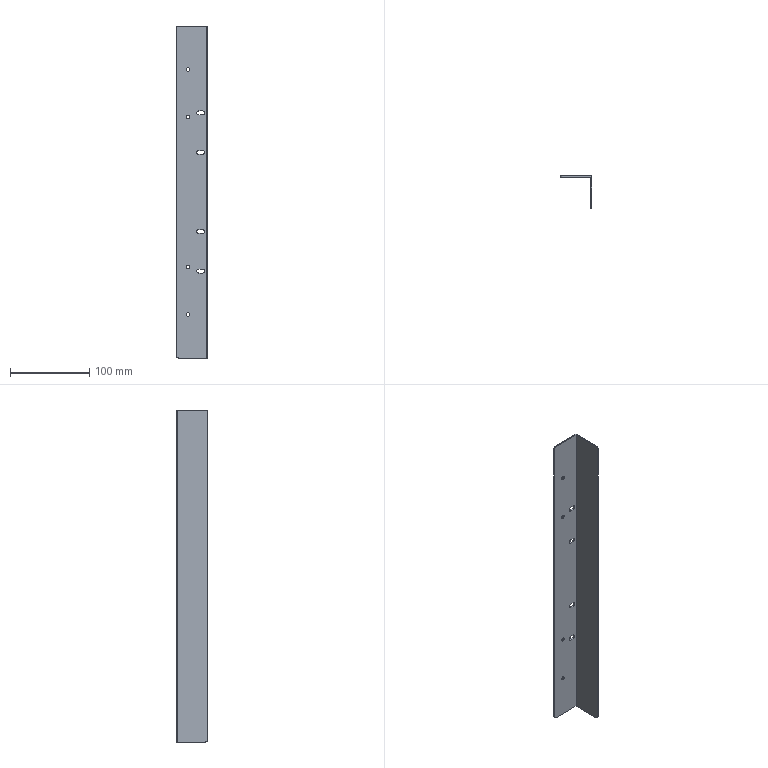Part | SolidWorks | features ICE 3, Cut 2, 3DProfileFeature 1, Extrusion 1, Fillet 1, HoleWzd 1 | 1 solid | 36 faces | box 40 x 40 x 420 mm | volume 49080 mm3 | cylinder 20 | plane 16 | commonest cylinder face diameters 4.5 x8 5 x8 6 x4
STEP:
#1=CARTESIAN_POINT('',(-23.5,20.,157.25));
#2=VERTEX_POINT('',#1);
#3=CARTESIAN_POINT('',(-23.5,20.,152.75));
#4=VERTEX_POINT('',#3);
#5=CARTESIAN_POINT('',(-23.5,20.,155.));
#6=DIRECTION('',(0.,-1.,0.));
#7=DIRECTION('',(0.,0.,-1.));
#8=AXIS2_PLACEMENT_3D('',#5,#6,#7);
#9=CIRCLE('',#8,2.25);
#10=EDGE_CURVE('',#2,#4,#9,.T.);
#11=ORIENTED_EDGE('',*,*,#10,.F.);
#12=CARTESIAN_POINT('',(-23.5,18.5,157.25));
#13=VERTEX_POINT('',#12);
#14=CARTESIAN_POINT('',(-23.5,28.5,157.25));
#15=DIRECTION('',(0.,-1.,0.));
#16=VECTOR('',#15,1000.);
#17=LINE('',#14,#16);
#18=EDGE_CURVE('',#2,#13,#17,.T.);
#19=ORIENTED_EDGE('',*,*,#18,.T.);
#20=CARTESIAN_POINT('',(-23.5,18.5,152.75));
#21=VERTEX_POINT('',#20);
#22=CARTESIAN_POINT('',(-23.5,18.5,155.));
#23=DIRECTION('',(0.,-1.,0.));
#24=DIRECTION('',(0.,0.,1.));
#25=AXIS2_PLACEMENT_3D('',#22,#23,#24);
#26=CIRCLE('',#25,2.25);
#27=EDGE_CURVE('',#13,#21,#26,.T.);
#28=ORIENTED_EDGE('',*,*,#27,.T.);
#29=CARTESIAN_POINT('',(-23.5,28.5,152.75));
#30=DIRECTION('',(0.,-1.,0.));
#31=VECTOR('',#30,1000.);
#32=LINE('',#29,#31);
#33=EDGE_CURVE('',#4,#21,#32,.T.);
#34=ORIENTED_EDGE('',*,*,#33,.F.);
#35=EDGE_LOOP('',(#11,#19,#28,#34));
#36=FACE_OUTER_BOUND('',#35,.T.);
#37=CARTESIAN_POINT('',(-23.5,28.5,155.));
#38=DIRECTION('',(0.,-1.,0.));
#39=DIRECTION('',(0.,0.,-1.));
#40=AXIS2_PLACEMENT_3D('',#37,#38,#39);
#41=CYLINDRICAL_SURFACE('',#40,2.25);
#42=ADVANCED_FACE('',(#36),#41,.F.);
#43=CARTESIAN_POINT('',(-23.5,20.,-152.75));
#44=VERTEX_POINT('',#43);
#45=CARTESIAN_POINT('',(-23.5,20.,-157.25));
#46=VERTEX_POINT('',#45);
#47=CARTESIAN_POINT('',(-23.5,20.,-155.));
#48=DIRECTION('',(0.,-1.,0.));
#49=DIRECTION('',(0.,0.,-1.));
#50=AXIS2_PLACEMENT_3D('',#47,#48,#49);
#51=CIRCLE('',#50,2.25);
#52=EDGE_CURVE('',#44,#46,#51,.T.);
#53=ORIENTED_EDGE('',*,*,#52,.F.);
#54=CARTESIAN_POINT('',(-23.5,18.5,-152.75));
#55=VERTEX_POINT('',#54);
#56=CARTESIAN_POINT('',(-23.5,28.5,-152.75));
#57=DIRECTION('',(0.,-1.,0.));
#58=VECTOR('',#57,1000.);
#59=LINE('',#56,#58);
#60=EDGE_CURVE('',#44,#55,#59,.T.);
#61=ORIENTED_EDGE('',*,*,#60,.T.);
#62=CARTESIAN_POINT('',(-23.5,18.5,-157.25));
#63=VERTEX_POINT('',#62);
#64=CARTESIAN_POINT('',(-23.5,18.5,-155.));
#65=DIRECTION('',(0.,-1.,0.));
#66=DIRECTION('',(0.,0.,-1.));
#67=AXIS2_PLACEMENT_3D('',#64,#65,#66);
#68=CIRCLE('',#67,2.25);
#69=EDGE_CURVE('',#55,#63,#68,.T.);
#70=ORIENTED_EDGE('',*,*,#69,.T.);
#71=CARTESIAN_POINT('',(-23.5,28.5,-157.25));
#72=DIRECTION('',(0.,-1.,0.));
#73=VECTOR('',#72,1000.);
#74=LINE('',#71,#73);
#75=EDGE_CURVE('',#46,#63,#74,.T.);
#76=ORIENTED_EDGE('',*,*,#75,.F.);
#77=EDGE_LOOP('',(#53,#61,#70,#76));
#78=FACE_OUTER_BOUND('',#77,.T.);
#79=CARTESIAN_POINT('',(-23.5,28.5,-155.));
#80=DIRECTION('',(0.,-1.,0.));
#81=DIRECTION('',(0.,0.,-1.));
#82=AXIS2_PLACEMENT_3D('',#79,#80,#81);
#83=CYLINDRICAL_SURFACE('',#82,2.25);
#84=ADVANCED_FACE('',(#78),#83,.F.);
#85=CARTESIAN_POINT('',(-23.5,18.5,-92.75));
#86=VERTEX_POINT('',#85);
#87=CARTESIAN_POINT('',(-23.5,18.5,-97.25));
#88=VERTEX_POINT('',#87);
#89=CARTESIAN_POINT('',(-23.5,18.5,-95.));
#90=DIRECTION('',(0.,-1.,0.));
#91=DIRECTION('',(0.,0.,-1.));
#92=AXIS2_PLACEMENT_3D('',#89,#90,#91);
#93=CIRCLE('',#92,2.25);
#94=EDGE_CURVE('',#86,#88,#93,.T.);
#95=ORIENTED_EDGE('',*,*,#94,.T.);
#96=CARTESIAN_POINT('',(-23.5,20.,-97.25));
#97=VERTEX_POINT('',#96);
#98=CARTESIAN_POINT('',(-23.5,10.,-97.25));
#99=DIRECTION('',(0.,1.,0.));
#100=VECTOR('',#99,1000.);
#101=LINE('',#98,#100);
#102=EDGE_CURVE('',#88,#97,#101,.T.);
#103=ORIENTED_EDGE('',*,*,#102,.T.);
#104=CARTESIAN_POINT('',(-23.5,20.,-92.75));
#105=VERTEX_POINT('',#104);
#106=CARTESIAN_POINT('',(-23.5,20.,-95.));
#107=DIRECTION('',(0.,1.,0.));
#108=DIRECTION('',(0.,0.,-1.));
#109=AXIS2_PLACEMENT_3D('',#106,#107,#108);
#110=CIRCLE('',#109,2.25);
#111=EDGE_CURVE('',#97,#105,#110,.T.);
#112=ORIENTED_EDGE('',*,*,#111,.T.);
#113=CARTESIAN_POINT('',(-23.5,10.,-92.75));
#114=DIRECTION('',(0.,1.,0.));
#115=VECTOR('',#114,1000.);
#116=LINE('',#113,#115);
#117=EDGE_CURVE('',#86,#105,#116,.T.);
#118=ORIENTED_EDGE('',*,*,#117,.F.);
#119=EDGE_LOOP('',(#95,#103,#112,#118));
#120=FACE_OUTER_BOUND('',#119,.T.);
#121=CARTESIAN_POINT('',(-23.5,10.,-95.));
#122=DIRECTION('',(0.,1.,0.));
#123=DIRECTION('',(0.,0.,1.));
#124=AXIS2_PLACEMENT_3D('',#121,#122,#123);
#125=CYLINDRICAL_SURFACE('',#124,2.25);
#126=ADVANCED_FACE('',(#120),#125,.F.);
#127=CARTESIAN_POINT('',(-23.5,18.5,97.25));
#128=VERTEX_POINT('',#127);
#129=CARTESIAN_POINT('',(-23.5,18.5,92.75));
#130=VERTEX_POINT('',#129);
#131=CARTESIAN_POINT('',(-23.5,18.5,95.));
#132=DIRECTION('',(0.,-1.,0.));
#133=DIRECTION('',(0.,0.,-1.));
#134=AXIS2_PLACEMENT_3D('',#131,#132,#133);
#135=CIRCLE('',#134,2.25);
#136=EDGE_CURVE('',#128,#130,#135,.T.);
#137=ORIENTED_EDGE('',*,*,#136,.T.);
#138=CARTESIAN_POINT('',(-23.5,20.,92.75));
#139=VERTEX_POINT('',#138);
#140=CARTESIAN_POINT('',(-23.5,10.,92.75));
#141=DIRECTION('',(0.,1.,0.));
#142=VECTOR('',#141,1000.);
#143=LINE('',#140,#142);
#144=EDGE_CURVE('',#130,#139,#143,.T.);
#145=ORIENTED_EDGE('',*,*,#144,.T.);
#146=CARTESIAN_POINT('',(-23.5,20.,97.25));
#147=VERTEX_POINT('',#146);
#148=CARTESIAN_POINT('',(-23.5,20.,95.));
#149=DIRECTION('',(0.,1.,0.));
#150=DIRECTION('',(0.,0.,1.));
#151=AXIS2_PLACEMENT_3D('',#148,#149,#150);
#152=CIRCLE('',#151,2.25);
#153=EDGE_CURVE('',#139,#147,#152,.T.);
#154=ORIENTED_EDGE('',*,*,#153,.T.);
#155=CARTESIAN_POINT('',(-23.5,10.,97.25));
#156=DIRECTION('',(0.,1.,0.));
#157=VECTOR('',#156,1000.);
#158=LINE('',#155,#157);
#159=EDGE_CURVE('',#128,#147,#158,.T.);
#160=ORIENTED_EDGE('',*,*,#159,.F.);
#161=EDGE_LOOP('',(#137,#145,#154,#160));
#162=FACE_OUTER_BOUND('',#161,.T.);
#163=CARTESIAN_POINT('',(-23.5,10.,95.));
#164=DIRECTION('',(0.,1.,0.));
#165=DIRECTION('',(0.,0.,1.));
#166=AXIS2_PLACEMENT_3D('',#163,#164,#165);
#167=CYLINDRICAL_SURFACE('',#166,2.25);
#168=ADVANCED_FACE('',(#162),#167,.F.);
#169=CARTESIAN_POINT('',(1.5,20.,210.));
#170=VERTEX_POINT('',#169);
#171=CARTESIAN_POINT('',(-35.5,20.,210.));
#172=VERTEX_POINT('',#171);
#173=CARTESIAN_POINT('',(1.5,20.,210.));
#174=DIRECTION('',(-1.,0.,0.));
#175=VECTOR('',#174,1000.);
#176=LINE('',#173,#175);
#177=EDGE_CURVE('',#170,#172,#176,.T.);
#178=ORIENTED_EDGE('',*,*,#177,.T.);
#179=CARTESIAN_POINT('',(-35.5,18.5,210.));
#180=VERTEX_POINT('',#179);
#181=CARTESIAN_POINT('',(-35.5,20.,210.));
#182=DIRECTION('',(0.,-1.,0.));
#183=VECTOR('',#182,1000.);
#184=LINE('',#181,#183);
#185=EDGE_CURVE('',#172,#180,#184,.T.);
#186=ORIENTED_EDGE('',*,*,#185,.T.);
#187=CARTESIAN_POINT('',(0.,18.5,210.));
#188=VERTEX_POINT('',#187);
#189=CARTESIAN_POINT('',(-38.5,18.5,210.));
#190=DIRECTION('',(1.,0.,0.));
#191=VECTOR('',#190,1000.);
#192=LINE('',#189,#191);
#193=EDGE_CURVE('',#180,#188,#192,.T.);
#194=ORIENTED_EDGE('',*,*,#193,.T.);
#195=CARTESIAN_POINT('',(0.,-17.,210.));
#196=VERTEX_POINT('',#195);
#197=CARTESIAN_POINT('',(0.,20.,210.));
#198=DIRECTION('',(0.,-1.,0.));
#199=VECTOR('',#198,1000.);
#200=LINE('',#197,#199);
#201=EDGE_CURVE('',#188,#196,#200,.T.);
#202=ORIENTED_EDGE('',*,*,#201,.T.);
#203=CARTESIAN_POINT('',(1.5,-17.,210.));
#204=VERTEX_POINT('',#203);
#205=CARTESIAN_POINT('',(1.5,-17.,210.));
#206=DIRECTION('',(1.,0.,0.));
#207=VECTOR('',#206,1000.);
#208=LINE('',#205,#207);
#209=EDGE_CURVE('',#196,#204,#208,.T.);
#210=ORIENTED_EDGE('',*,*,#209,.T.);
#211=CARTESIAN_POINT('',(1.5,20.,210.));
#212=DIRECTION('',(0.,-1.,0.));
#213=VECTOR('',#212,1000.);
#214=LINE('',#211,#213);
#215=EDGE_CURVE('',#170,#204,#214,.T.);
#216=ORIENTED_EDGE('',*,*,#215,.F.);
#217=EDGE_LOOP('',(#178,#186,#194,#202,#210,#216));
#218=FACE_OUTER_BOUND('',#217,.T.);
#219=CARTESIAN_POINT('',(1.5,20.,210.));
#220=DIRECTION('',(0.,0.,-1.));
#221=DIRECTION('',(-1.,0.,0.));
#222=AXIS2_PLACEMENT_3D('',#219,#220,#221);
#223=PLANE('',#222);
#224=ADVANCED_FACE('',(#218),#223,.F.);
#225=CARTESIAN_POINT('',(1.5,-20.,207.));
#226=VERTEX_POINT('',#225);
#227=CARTESIAN_POINT('',(1.5,-20.,-207.));
#228=VERTEX_POINT('',#227);
#229=CARTESIAN_POINT('',(1.5,-20.,210.));
#230=DIRECTION('',(0.,0.,-1.));
#231=VECTOR('',#230,1000.);
#232=LINE('',#229,#231);
#233=EDGE_CURVE('',#226,#228,#232,.T.);
#234=ORIENTED_EDGE('',*,*,#233,.F.);
#235=CARTESIAN_POINT('',(0.,-20.,207.));
#236=VERTEX_POINT('',#235);
#237=CARTESIAN_POINT('',(1.5,-20.,207.));
#238=DIRECTION('',(-1.,0.,0.));
#239=VECTOR('',#238,1000.);
#240=LINE('',#237,#239);
#241=EDGE_CURVE('',#226,#236,#240,.T.);
#242=ORIENTED_EDGE('',*,*,#241,.T.);
#243=CARTESIAN_POINT('',(0.,-20.,-207.));
#244=VERTEX_POINT('',#243);
#245=CARTESIAN_POINT('',(0.,-20.,210.));
#246=DIRECTION('',(0.,0.,-1.));
#247=VECTOR('',#246,1000.);
#248=LINE('',#245,#247);
#249=EDGE_CURVE('',#236,#244,#248,.T.);
#250=ORIENTED_EDGE('',*,*,#249,.T.);
#251=CARTESIAN_POINT('',(1.5,-20.,-207.));
#252=DIRECTION('',(1.,0.,0.));
#253=VECTOR('',#252,1000.);
#254=LINE('',#251,#253);
#255=EDGE_CURVE('',#244,#228,#254,.T.);
#256=ORIENTED_EDGE('',*,*,#255,.T.);
#257=EDGE_LOOP('',(#234,#242,#250,#256));
#258=FACE_OUTER_BOUND('',#257,.T.);
#259=CARTESIAN_POINT('',(1.5,-20.,210.));
#260=DIRECTION('',(0.,1.,0.));
#261=DIRECTION('',(0.,0.,1.));
#262=AXIS2_PLACEMENT_3D('',#259,#260,#261);
#263=PLANE('',#262);
#264=ADVANCED_FACE('',(#258),#263,.F.);
#265=CARTESIAN_POINT('',(-35.5,18.5,-210.));
#266=VERTEX_POINT('',#265);
#267=CARTESIAN_POINT('',(0.,18.5,-210.));
#268=VERTEX_POINT('',#267);
#269=CARTESIAN_POINT('',(-38.5,18.5,-210.));
#270=DIRECTION('',(1.,0.,0.));
#271=VECTOR('',#270,1000.);
#272=LINE('',#269,#271);
#273=EDGE_CURVE('',#266,#268,#272,.T.);
#274=ORIENTED_EDGE('',*,*,#273,.F.);
#275=CARTESIAN_POINT('',(-35.5,20.,-210.));
#276=VERTEX_POINT('',#275);
#277=CARTESIAN_POINT('',(-35.5,20.,-210.));
#278=DIRECTION('',(0.,1.,0.));
#279=VECTOR('',#278,1000.);
#280=LINE('',#277,#279);
#281=EDGE_CURVE('',#266,#276,#280,.T.);
#282=ORIENTED_EDGE('',*,*,#281,.T.);
#283=CARTESIAN_POINT('',(1.5,20.,-210.));
#284=VERTEX_POINT('',#283);
#285=CARTESIAN_POINT('',(1.5,20.,-210.));
#286=DIRECTION('',(-1.,0.,0.));
#287=VECTOR('',#286,1000.);
#288=LINE('',#285,#287);
#289=EDGE_CURVE('',#284,#276,#288,.T.);
#290=ORIENTED_EDGE('',*,*,#289,.F.);
#291=CARTESIAN_POINT('',(1.5,-17.,-210.));
#292=VERTEX_POINT('',#291);
#293=CARTESIAN_POINT('',(1.5,20.,-210.));
#294=DIRECTION('',(0.,1.,0.));
#295=VECTOR('',#294,1000.);
#296=LINE('',#293,#295);
#297=EDGE_CURVE('',#292,#284,#296,.T.);
#298=ORIENTED_EDGE('',*,*,#297,.F.);
#299=CARTESIAN_POINT('',(0.,-17.,-210.));
#300=VERTEX_POINT('',#299);
#301=CARTESIAN_POINT('',(1.5,-17.,-210.));
#302=DIRECTION('',(-1.,0.,0.));
#303=VECTOR('',#302,1000.);
#304=LINE('',#301,#303);
#305=EDGE_CURVE('',#292,#300,#304,.T.);
#306=ORIENTED_EDGE('',*,*,#305,.T.);
#307=CARTESIAN_POINT('',(0.,20.,-210.));
#308=DIRECTION('',(0.,1.,0.));
#309=VECTOR('',#308,1000.);
#310=LINE('',#307,#309);
#311=EDGE_CURVE('',#300,#268,#310,.T.);
#312=ORIENTED_EDGE('',*,*,#311,.T.);
#313=EDGE_LOOP('',(#274,#282,#290,#298,#306,#312));
#314=FACE_OUTER_BOUND('',#313,.T.);
#315=CARTESIAN_POINT('',(1.5,20.,-210.));
#316=DIRECTION('',(0.,0.,1.));
#317=DIRECTION('',(1.,0.,0.));
#318=AXIS2_PLACEMENT_3D('',#315,#316,#317);
#319=PLANE('',#318);
#320=ADVANCED_FACE('',(#314),#319,.F.);
#321=CARTESIAN_POINT('',(-5.,20.,-102.5));
#322=VERTEX_POINT('',#321);
#323=CARTESIAN_POINT('',(-10.,20.,-102.5));
#324=VERTEX_POINT('',#323);
#325=CARTESIAN_POINT('',(-5.,20.,-102.5));
#326=DIRECTION('',(-1.,0.,0.));
#327=VECTOR('',#326,1000.);
#328=LINE('',#325,#327);
#329=EDGE_CURVE('',#322,#324,#328,.T.);
#330=ORIENTED_EDGE('',*,*,#329,.F.);
#331=CARTESIAN_POINT('',(-5.,20.,-97.5));
#332=VERTEX_POINT('',#331);
#333=CARTESIAN_POINT('',(-5.,20.,-100.));
#334=DIRECTION('',(0.,1.,0.));
#335=DIRECTION('',(0.,0.,1.));
#336=AXIS2_PLACEMENT_3D('',#333,#334,#335);
#337=CIRCLE('',#336,2.5);
#338=EDGE_CURVE('',#332,#322,#337,.T.);
#339=ORIENTED_EDGE('',*,*,#338,.F.);
#340=CARTESIAN_POINT('',(-10.,20.,-97.5));
#341=VERTEX_POINT('',#340);
#342=CARTESIAN_POINT('',(-5.,20.,-97.5));
#343=DIRECTION('',(1.,0.,0.));
#344=VECTOR('',#343,1000.);
#345=LINE('',#342,#344);
#346=EDGE_CURVE('',#341,#332,#345,.T.);
#347=ORIENTED_EDGE('',*,*,#346,.F.);
#348=CARTESIAN_POINT('',(-10.,20.,-100.));
#349=DIRECTION('',(0.,1.,0.));
#350=DIRECTION('',(0.,0.,1.));
#351=AXIS2_PLACEMENT_3D('',#348,#349,#350);
#352=CIRCLE('',#351,2.5);
#353=EDGE_CURVE('',#324,#341,#352,.T.);
#354=ORIENTED_EDGE('',*,*,#353,.F.);
#355=EDGE_LOOP('',(#330,#339,#347,#354));
#356=FACE_BOUND('',#355,.T.);
#357=CARTESIAN_POINT('',(-5.,20.,47.5));
#358=VERTEX_POINT('',#357);
#359=CARTESIAN_POINT('',(-10.,20.,47.5));
#360=VERTEX_POINT('',#359);
#361=CARTESIAN_POINT('',(-5.,20.,47.5));
#362=DIRECTION('',(-1.,0.,0.));
#363=VECTOR('',#362,1000.);
#364=LINE('',#361,#363);
#365=EDGE_CURVE('',#358,#360,#364,.T.);
#366=ORIENTED_EDGE('',*,*,#365,.F.);
#367=CARTESIAN_POINT('',(-5.,20.,52.5));
#368=VERTEX_POINT('',#367);
#369=CARTESIAN_POINT('',(-5.,20.,50.));
#370=DIRECTION('',(0.,1.,0.));
#371=DIRECTION('',(0.,0.,1.));
#372=AXIS2_PLACEMENT_3D('',#369,#370,#371);
#373=CIRCLE('',#372,2.5);
#374=EDGE_CURVE('',#368,#358,#373,.T.);
#375=ORIENTED_EDGE('',*,*,#374,.F.);
#376=CARTESIAN_POINT('',(-10.,20.,52.5));
#377=VERTEX_POINT('',#376);
#378=CARTESIAN_POINT('',(-5.,20.,52.5));
#379=DIRECTION('',(1.,0.,0.));
#380=VECTOR('',#379,1000.);
#381=LINE('',#378,#380);
#382=EDGE_CURVE('',#377,#368,#381,.T.);
#383=ORIENTED_EDGE('',*,*,#382,.F.);
#384=CARTESIAN_POINT('',(-10.,20.,50.));
#385=DIRECTION('',(0.,1.,0.));
#386=DIRECTION('',(0.,0.,1.));
#387=AXIS2_PLACEMENT_3D('',#384,#385,#386);
#388=CIRCLE('',#387,2.5);
#389=EDGE_CURVE('',#360,#377,#388,.T.);
#390=ORIENTED_EDGE('',*,*,#389,.F.);
#391=EDGE_LOOP('',(#366,#375,#383,#390));
#392=FACE_BOUND('',#391,.T.);
#393=CARTESIAN_POINT('',(-5.,20.,-52.5));
#394=VERTEX_POINT('',#393);
#395=CARTESIAN_POINT('',(-10.,20.,-52.5));
#396=VERTEX_POINT('',#395);
#397=CARTESIAN_POINT('',(-5.,20.,-52.5));
#398=DIRECTION('',(-1.,0.,0.));
#399=VECTOR('',#398,1000.);
#400=LINE('',#397,#399);
#401=EDGE_CURVE('',#394,#396,#400,.T.);
#402=ORIENTED_EDGE('',*,*,#401,.F.);
#403=CARTESIAN_POINT('',(-5.,20.,-47.5));
#404=VERTEX_POINT('',#403);
#405=CARTESIAN_POINT('',(-5.,20.,-50.));
#406=DIRECTION('',(0.,1.,0.));
#407=DIRECTION('',(0.,0.,1.));
#408=AXIS2_PLACEMENT_3D('',#405,#406,#407);
#409=CIRCLE('',#408,2.5);
#410=EDGE_CURVE('',#404,#394,#409,.T.);
#411=ORIENTED_EDGE('',*,*,#410,.F.);
#412=CARTESIAN_POINT('',(-10.,20.,-47.5));
#413=VERTEX_POINT('',#412);
#414=CARTESIAN_POINT('',(-5.,20.,-47.5));
#415=DIRECTION('',(1.,0.,0.));
#416=VECTOR('',#415,1000.);
#417=LINE('',#414,#416);
#418=EDGE_CURVE('',#413,#404,#417,.T.);
#419=ORIENTED_EDGE('',*,*,#418,.F.);
#420=CARTESIAN_POINT('',(-10.,20.,-50.));
#421=DIRECTION('',(0.,1.,0.));
#422=DIRECTION('',(0.,0.,1.));
#423=AXIS2_PLACEMENT_3D('',#420,#421,#422);
#424=CIRCLE('',#423,2.5);
#425=EDGE_CURVE('',#396,#413,#424,.T.);
#426=ORIENTED_EDGE('',*,*,#425,.F.);
#427=EDGE_LOOP('',(#402,#411,#419,#426));
#428=FACE_BOUND('',#427,.T.);
#429=CARTESIAN_POINT('',(-10.,20.,102.5));
#430=VERTEX_POINT('',#429);
#431=CARTESIAN_POINT('',(-5.,20.,102.5));
#432=VERTEX_POINT('',#431);
#433=CARTESIAN_POINT('',(-10.,20.,102.5));
#434=DIRECTION('',(1.,0.,0.));
#435=VECTOR('',#434,1000.);
#436=LINE('',#433,#435);
#437=EDGE_CURVE('',#430,#432,#436,.T.);
#438=ORIENTED_EDGE('',*,*,#437,.F.);
#439=CARTESIAN_POINT('',(-10.,20.,97.5));
#440=VERTEX_POINT('',#439);
#441=CARTESIAN_POINT('',(-10.,20.,100.));
#442=DIRECTION('',(0.,1.,0.));
#443=DIRECTION('',(0.,0.,1.));
#444=AXIS2_PLACEMENT_3D('',#441,#442,#443);
#445=CIRCLE('',#444,2.5);
#446=EDGE_CURVE('',#440,#430,#445,.T.);
#447=ORIENTED_EDGE('',*,*,#446,.F.);
#448=CARTESIAN_POINT('',(-5.,20.,97.5));
#449=VERTEX_POINT('',#448);
#450=CARTESIAN_POINT('',(-10.,20.,97.5));
#451=DIRECTION('',(-1.,0.,0.));
#452=VECTOR('',#451,1000.);
#453=LINE('',#450,#452);
#454=EDGE_CURVE('',#449,#440,#453,.T.);
#455=ORIENTED_EDGE('',*,*,#454,.F.);
#456=CARTESIAN_POINT('',(-5.,20.,100.));
#457=DIRECTION('',(0.,1.,0.));
#458=DIRECTION('',(0.,0.,1.));
#459=AXIS2_PLACEMENT_3D('',#456,#457,#458);
#460=CIRCLE('',#459,2.5);
#461=EDGE_CURVE('',#432,#449,#460,.T.);
#462=ORIENTED_EDGE('',*,*,#461,.F.);
#463=EDGE_LOOP('',(#438,#447,#455,#462));
#464=FACE_BOUND('',#463,.T.);
#465=CARTESIAN_POINT('',(-23.5,20.,155.));
#466=DIRECTION('',(0.,-1.,0.));
#467=DIRECTION('',(0.,0.,-1.));
#468=AXIS2_PLACEMENT_3D('',#465,#466,#467);
#469=CIRCLE('',#468,2.25);
#470=EDGE_CURVE('',#4,#2,#469,.T.);
#471=ORIENTED_EDGE('',*,*,#470,.T.);
#472=ORIENTED_EDGE('',*,*,#10,.T.);
#473=EDGE_LOOP('',(#471,#472));
#474=FACE_BOUND('',#473,.T.);
#475=CARTESIAN_POINT('',(-23.5,20.,-155.));
#476=DIRECTION('',(0.,-1.,0.));
#477=DIRECTION('',(0.,0.,-1.));
#478=AXIS2_PLACEMENT_3D('',#475,#476,#477);
#479=CIRCLE('',#478,2.25);
#480=EDGE_CURVE('',#46,#44,#479,.T.);
#481=ORIENTED_EDGE('',*,*,#480,.T.);
#482=ORIENTED_EDGE('',*,*,#52,.T.);
#483=EDGE_LOOP('',(#481,#482));
#484=FACE_BOUND('',#483,.T.);
#485=CARTESIAN_POINT('',(-23.5,20.,-95.));
#486=DIRECTION('',(0.,1.,0.));
#487=DIRECTION('',(0.,0.,-1.));
#488=AXIS2_PLACEMENT_3D('',#485,#486,#487);
#489=CIRCLE('',#488,2.25);
#490=EDGE_CURVE('',#105,#97,#489,.T.);
#491=ORIENTED_EDGE('',*,*,#490,.F.);
#492=ORIENTED_EDGE('',*,*,#111,.F.);
#493=EDGE_LOOP('',(#491,#492));
#494=FACE_BOUND('',#493,.T.);
#495=CARTESIAN_POINT('',(-23.5,20.,95.));
#496=DIRECTION('',(0.,1.,0.));
#497=DIRECTION('',(0.,0.,1.));
#498=AXIS2_PLACEMENT_3D('',#495,#496,#497);
#499=CIRCLE('',#498,2.25);
#500=EDGE_CURVE('',#147,#139,#499,.T.);
#501=ORIENTED_EDGE('',*,*,#500,.F.);
#502=ORIENTED_EDGE('',*,*,#153,.F.);
#503=EDGE_LOOP('',(#501,#502));
#504=FACE_BOUND('',#503,.T.);
#505=CARTESIAN_POINT('',(-38.5,20.,-207.));
#506=VERTEX_POINT('',#505);
#507=CARTESIAN_POINT('',(-38.5,20.,207.));
#508=VERTEX_POINT('',#507);
#509=CARTESIAN_POINT('',(-38.5,20.,210.));
#510=DIRECTION('',(0.,0.,1.));
#511=VECTOR('',#510,1000.);
#512=LINE('',#509,#511);
#513=EDGE_CURVE('',#506,#508,#512,.T.);
#514=ORIENTED_EDGE('',*,*,#513,.T.);
#515=CARTESIAN_POINT('',(-35.5,20.,207.));
#516=DIRECTION('',(0.,1.,0.));
#517=DIRECTION('',(0.,0.,-1.));
#518=AXIS2_PLACEMENT_3D('',#515,#516,#517);
#519=CIRCLE('',#518,3.);
#520=EDGE_CURVE('',#508,#172,#519,.T.);
#521=ORIENTED_EDGE('',*,*,#520,.T.);
#522=ORIENTED_EDGE('',*,*,#177,.F.);
#523=CARTESIAN_POINT('',(1.5,20.,210.));
#524=DIRECTION('',(0.,0.,1.));
#525=VECTOR('',#524,1000.);
#526=LINE('',#523,#525);
#527=EDGE_CURVE('',#284,#170,#526,.T.);
#528=ORIENTED_EDGE('',*,*,#527,.F.);
#529=ORIENTED_EDGE('',*,*,#289,.T.);
#530=CARTESIAN_POINT('',(-35.5,20.,-207.));
#531=DIRECTION('',(0.,1.,0.));
#532=DIRECTION('',(0.,0.,-1.));
#533=AXIS2_PLACEMENT_3D('',#530,#531,#532);
#534=CIRCLE('',#533,3.);
#535=EDGE_CURVE('',#276,#506,#534,.T.);
#536=ORIENTED_EDGE('',*,*,#535,.T.);
#537=EDGE_LOOP('',(#514,#521,#522,#528,#529,#536));
#538=FACE_OUTER_BOUND('',#537,.T.);
#539=CARTESIAN_POINT('',(1.5,20.,210.));
#540=DIRECTION('',(0.,-1.,0.));
#541=DIRECTION('',(0.,0.,-1.));
#542=AXIS2_PLACEMENT_3D('',#539,#540,#541);
#543=PLANE('',#542);
#544=ADVANCED_FACE('',(#356,#392,#428,#464,#474,#484,#494,#504,#538),#543,.F.);
#545=ORIENTED_EDGE('',*,*,#215,.T.);
#546=CARTESIAN_POINT('',(1.5,-17.,207.));
#547=DIRECTION('',(1.,0.,0.));
#548=DIRECTION('',(0.,0.,-1.));
#549=AXIS2_PLACEMENT_3D('',#546,#547,#548);
#550=CIRCLE('',#549,3.);
#551=EDGE_CURVE('',#204,#226,#550,.T.);
#552=ORIENTED_EDGE('',*,*,#551,.T.);
#553=ORIENTED_EDGE('',*,*,#233,.T.);
#554=CARTESIAN_POINT('',(1.5,-17.,-207.));
#555=DIRECTION('',(1.,0.,0.));
#556=DIRECTION('',(0.,0.,-1.));
#557=AXIS2_PLACEMENT_3D('',#554,#555,#556);
#558=CIRCLE('',#557,3.);
#559=EDGE_CURVE('',#228,#292,#558,.T.);
#560=ORIENTED_EDGE('',*,*,#559,.T.);
#561=ORIENTED_EDGE('',*,*,#297,.T.);
#562=ORIENTED_EDGE('',*,*,#527,.T.);
#563=EDGE_LOOP('',(#545,#552,#553,#560,#561,#562));
#564=FACE_OUTER_BOUND('',#563,.T.);
#565=CARTESIAN_POINT('',(1.5,-20.,210.));
#566=DIRECTION('',(1.,0.,0.));
#567=DIRECTION('',(0.,0.,-1.));
#568=AXIS2_PLACEMENT_3D('',#565,#566,#567);
#569=PLANE('',#568);
#570=ADVANCED_FACE('',(#564),#569,.T.);
#571=ORIENTED_EDGE('',*,*,#249,.F.);
#572=CARTESIAN_POINT('',(0.,-17.,207.));
#573=DIRECTION('',(-1.,0.,0.));
#574=DIRECTION('',(0.,0.,-1.));
#575=AXIS2_PLACEMENT_3D('',#572,#573,#574);
#576=CIRCLE('',#575,3.);
#577=EDGE_CURVE('',#236,#196,#576,.T.);
#578=ORIENTED_EDGE('',*,*,#577,.T.);
#579=ORIENTED_EDGE('',*,*,#201,.F.);
#580=CARTESIAN_POINT('',(0.,18.5,210.));
#581=DIRECTION('',(0.,0.,-1.));
#582=VECTOR('',#581,1000.);
#583=LINE('',#580,#582);
#584=EDGE_CURVE('',#188,#268,#583,.T.);
#585=ORIENTED_EDGE('',*,*,#584,.T.);
#586=ORIENTED_EDGE('',*,*,#311,.F.);
#587=CARTESIAN_POINT('',(0.,-17.,-207.));
#588=DIRECTION('',(-1.,0.,0.));
#589=DIRECTION('',(0.,0.,-1.));
#590=AXIS2_PLACEMENT_3D('',#587,#588,#589);
#591=CIRCLE('',#590,3.);
#592=EDGE_CURVE('',#300,#244,#591,.T.);
#593=ORIENTED_EDGE('',*,*,#592,.T.);
#594=EDGE_LOOP('',(#571,#578,#579,#585,#586,#593));
#595=FACE_OUTER_BOUND('',#594,.T.);
#596=CARTESIAN_POINT('',(0.,-20.,210.));
#597=DIRECTION('',(1.,0.,0.));
#598=DIRECTION('',(0.,0.,-1.));
#599=AXIS2_PLACEMENT_3D('',#596,#597,#598);
#600=PLANE('',#599);
#601=ADVANCED_FACE('',(#595),#600,.F.);
#602=CARTESIAN_POINT('',(-5.,18.5,-102.5));
#603=VERTEX_POINT('',#602);
#604=CARTESIAN_POINT('',(-5.,18.5,-97.5));
#605=VERTEX_POINT('',#604);
#606=CARTESIAN_POINT('',(-5.,18.5,-100.));
#607=DIRECTION('',(0.,-1.,0.));
#608=DIRECTION('',(0.,0.,-1.));
#609=AXIS2_PLACEMENT_3D('',#606,#607,#608);
#610=CIRCLE('',#609,2.5);
#611=EDGE_CURVE('',#603,#605,#610,.T.);
#612=ORIENTED_EDGE('',*,*,#611,.F.);
#613=CARTESIAN_POINT('',(-10.,18.5,-102.5));
#614=VERTEX_POINT('',#613);
#615=CARTESIAN_POINT('',(-38.5,18.5,-102.5));
#616=DIRECTION('',(1.,0.,0.));
#617=VECTOR('',#616,1000.);
#618=LINE('',#615,#617);
#619=EDGE_CURVE('',#614,#603,#618,.T.);
#620=ORIENTED_EDGE('',*,*,#619,.F.);
#621=CARTESIAN_POINT('',(-10.,18.5,-97.5));
#622=VERTEX_POINT('',#621);
#623=CARTESIAN_POINT('',(-10.,18.5,-100.));
#624=DIRECTION('',(0.,-1.,0.));
#625=DIRECTION('',(0.,0.,-1.));
#626=AXIS2_PLACEMENT_3D('',#623,#624,#625);
#627=CIRCLE('',#626,2.5);
#628=EDGE_CURVE('',#622,#614,#627,.T.);
#629=ORIENTED_EDGE('',*,*,#628,.F.);
#630=CARTESIAN_POINT('',(-38.5,18.5,-97.5));
#631=DIRECTION('',(-1.,0.,0.));
#632=VECTOR('',#631,1000.);
#633=LINE('',#630,#632);
#634=EDGE_CURVE('',#605,#622,#633,.T.);
#635=ORIENTED_EDGE('',*,*,#634,.F.);
#636=EDGE_LOOP('',(#612,#620,#629,#635));
#637=FACE_BOUND('',#636,.T.);
#638=CARTESIAN_POINT('',(-5.,18.5,47.5));
#639=VERTEX_POINT('',#638);
#640=CARTESIAN_POINT('',(-5.,18.5,52.5));
#641=VERTEX_POINT('',#640);
#642=CARTESIAN_POINT('',(-5.,18.5,50.));
#643=DIRECTION('',(0.,-1.,0.));
#644=DIRECTION('',(0.,0.,-1.));
#645=AXIS2_PLACEMENT_3D('',#642,#643,#644);
#646=CIRCLE('',#645,2.5);
#647=EDGE_CURVE('',#639,#641,#646,.T.);
#648=ORIENTED_EDGE('',*,*,#647,.F.);
#649=CARTESIAN_POINT('',(-10.,18.5,47.5));
#650=VERTEX_POINT('',#649);
#651=CARTESIAN_POINT('',(-38.5,18.5,47.5));
#652=DIRECTION('',(1.,0.,0.));
#653=VECTOR('',#652,1000.);
#654=LINE('',#651,#653);
#655=EDGE_CURVE('',#650,#639,#654,.T.);
#656=ORIENTED_EDGE('',*,*,#655,.F.);
#657=CARTESIAN_POINT('',(-10.,18.5,52.5));
#658=VERTEX_POINT('',#657);
#659=CARTESIAN_POINT('',(-10.,18.5,50.));
#660=DIRECTION('',(0.,-1.,0.));
#661=DIRECTION('',(0.,0.,-1.));
#662=AXIS2_PLACEMENT_3D('',#659,#660,#661);
#663=CIRCLE('',#662,2.5);
#664=EDGE_CURVE('',#658,#650,#663,.T.);
#665=ORIENTED_EDGE('',*,*,#664,.F.);
#666=CARTESIAN_POINT('',(-38.5,18.5,52.5));
#667=DIRECTION('',(-1.,0.,0.));
#668=VECTOR('',#667,1000.);
#669=LINE('',#666,#668);
#670=EDGE_CURVE('',#641,#658,#669,.T.);
#671=ORIENTED_EDGE('',*,*,#670,.F.);
#672=EDGE_LOOP('',(#648,#656,#665,#671));
#673=FACE_BOUND('',#672,.T.);
#674=CARTESIAN_POINT('',(-5.,18.5,-52.5));
#675=VERTEX_POINT('',#674);
#676=CARTESIAN_POINT('',(-5.,18.5,-47.5));
#677=VERTEX_POINT('',#676);
#678=CARTESIAN_POINT('',(-5.,18.5,-50.));
#679=DIRECTION('',(0.,-1.,0.));
#680=DIRECTION('',(0.,0.,-1.));
#681=AXIS2_PLACEMENT_3D('',#678,#679,#680);
#682=CIRCLE('',#681,2.5);
#683=EDGE_CURVE('',#675,#677,#682,.T.);
#684=ORIENTED_EDGE('',*,*,#683,.F.);
#685=CARTESIAN_POINT('',(-10.,18.5,-52.5));
#686=VERTEX_POINT('',#685);
#687=CARTESIAN_POINT('',(-38.5,18.5,-52.5));
#688=DIRECTION('',(1.,0.,0.));
#689=VECTOR('',#688,1000.);
#690=LINE('',#687,#689);
#691=EDGE_CURVE('',#686,#675,#690,.T.);
#692=ORIENTED_EDGE('',*,*,#691,.F.);
#693=CARTESIAN_POINT('',(-10.,18.5,-47.5));
#694=VERTEX_POINT('',#693);
#695=CARTESIAN_POINT('',(-10.,18.5,-50.));
#696=DIRECTION('',(0.,-1.,0.));
#697=DIRECTION('',(0.,0.,-1.));
#698=AXIS2_PLACEMENT_3D('',#695,#696,#697);
#699=CIRCLE('',#698,2.5);
#700=EDGE_CURVE('',#694,#686,#699,.T.);
#701=ORIENTED_EDGE('',*,*,#700,.F.);
#702=CARTESIAN_POINT('',(-38.5,18.5,-47.5));
#703=DIRECTION('',(-1.,0.,0.));
#704=VECTOR('',#703,1000.);
#705=LINE('',#702,#704);
#706=EDGE_CURVE('',#677,#694,#705,.T.);
#707=ORIENTED_EDGE('',*,*,#706,.F.);
#708=EDGE_LOOP('',(#684,#692,#701,#707));
#709=FACE_BOUND('',#708,.T.);
#710=CARTESIAN_POINT('',(-10.,18.5,102.5));
#711=VERTEX_POINT('',#710);
#712=CARTESIAN_POINT('',(-10.,18.5,97.5));
#713=VERTEX_POINT('',#712);
#714=CARTESIAN_POINT('',(-10.,18.5,100.));
#715=DIRECTION('',(0.,-1.,0.));
#716=DIRECTION('',(0.,0.,-1.));
#717=AXIS2_PLACEMENT_3D('',#714,#715,#716);
#718=CIRCLE('',#717,2.5);
#719=EDGE_CURVE('',#711,#713,#718,.T.);
#720=ORIENTED_EDGE('',*,*,#719,.F.);
#721=CARTESIAN_POINT('',(-5.,18.5,102.5));
#722=VERTEX_POINT('',#721);
#723=CARTESIAN_POINT('',(-38.5,18.5,102.5));
#724=DIRECTION('',(-1.,0.,0.));
#725=VECTOR('',#724,1000.);
#726=LINE('',#723,#725);
#727=EDGE_CURVE('',#722,#711,#726,.T.);
#728=ORIENTED_EDGE('',*,*,#727,.F.);
#729=CARTESIAN_POINT('',(-5.,18.5,97.5));
#730=VERTEX_POINT('',#729);
#731=CARTESIAN_POINT('',(-5.,18.5,100.));
#732=DIRECTION('',(0.,-1.,0.));
#733=DIRECTION('',(0.,0.,-1.));
#734=AXIS2_PLACEMENT_3D('',#731,#732,#733);
#735=CIRCLE('',#734,2.5);
#736=EDGE_CURVE('',#730,#722,#735,.T.);
#737=ORIENTED_EDGE('',*,*,#736,.F.);
#738=CARTESIAN_POINT('',(-38.5,18.5,97.5));
#739=DIRECTION('',(1.,0.,0.));
#740=VECTOR('',#739,1000.);
#741=LINE('',#738,#740);
#742=EDGE_CURVE('',#713,#730,#741,.T.);
#743=ORIENTED_EDGE('',*,*,#742,.F.);
#744=EDGE_LOOP('',(#720,#728,#737,#743));
#745=FACE_BOUND('',#744,.T.);
#746=CARTESIAN_POINT('',(-23.5,18.5,155.));
#747=DIRECTION('',(0.,-1.,0.));
#748=DIRECTION('',(0.,0.,1.));
#749=AXIS2_PLACEMENT_3D('',#746,#747,#748);
#750=CIRCLE('',#749,2.25);
#751=EDGE_CURVE('',#21,#13,#750,.T.);
#752=ORIENTED_EDGE('',*,*,#751,.F.);
#753=ORIENTED_EDGE('',*,*,#27,.F.);
#754=EDGE_LOOP('',(#752,#753));
#755=FACE_BOUND('',#754,.T.);
#756=CARTESIAN_POINT('',(-23.5,18.5,-155.));
#757=DIRECTION('',(0.,-1.,0.));
#758=DIRECTION('',(0.,0.,-1.));
#759=AXIS2_PLACEMENT_3D('',#756,#757,#758);
#760=CIRCLE('',#759,2.25);
#761=EDGE_CURVE('',#63,#55,#760,.T.);
#762=ORIENTED_EDGE('',*,*,#761,.F.);
#763=ORIENTED_EDGE('',*,*,#69,.F.);
#764=EDGE_LOOP('',(#762,#763));
#765=FACE_BOUND('',#764,.T.);
#766=ORIENTED_EDGE('',*,*,#94,.F.);
#767=CARTESIAN_POINT('',(-23.5,18.5,-95.));
#768=DIRECTION('',(0.,-1.,0.));
#769=DIRECTION('',(0.,0.,-1.));
#770=AXIS2_PLACEMENT_3D('',#767,#768,#769);
#771=CIRCLE('',#770,2.25);
#772=EDGE_CURVE('',#88,#86,#771,.T.);
#773=ORIENTED_EDGE('',*,*,#772,.F.);
#774=EDGE_LOOP('',(#766,#773));
#775=FACE_BOUND('',#774,.T.);
#776=ORIENTED_EDGE('',*,*,#136,.F.);
#777=CARTESIAN_POINT('',(-23.5,18.5,95.));
#778=DIRECTION('',(0.,-1.,0.));
#779=DIRECTION('',(0.,0.,-1.));
#780=AXIS2_PLACEMENT_3D('',#777,#778,#779);
#781=CIRCLE('',#780,2.25);
#782=EDGE_CURVE('',#130,#128,#781,.T.);
#783=ORIENTED_EDGE('',*,*,#782,.F.);
#784=EDGE_LOOP('',(#776,#783));
#785=FACE_BOUND('',#784,.T.);
#786=ORIENTED_EDGE('',*,*,#193,.F.);
#787=CARTESIAN_POINT('',(-38.5,18.5,207.));
#788=VERTEX_POINT('',#787);
#789=CARTESIAN_POINT('',(-35.5,18.5,207.));
#790=DIRECTION('',(0.,-1.,0.));
#791=DIRECTION('',(0.,0.,-1.));
#792=AXIS2_PLACEMENT_3D('',#789,#790,#791);
#793=CIRCLE('',#792,3.);
#794=EDGE_CURVE('',#180,#788,#793,.T.);
#795=ORIENTED_EDGE('',*,*,#794,.T.);
#796=CARTESIAN_POINT('',(-38.5,18.5,-207.));
#797=VERTEX_POINT('',#796);
#798=CARTESIAN_POINT('',(-38.5,18.5,210.));
#799=DIRECTION('',(0.,0.,-1.));
#800=VECTOR('',#799,1000.);
#801=LINE('',#798,#800);
#802=EDGE_CURVE('',#788,#797,#801,.T.);
#803=ORIENTED_EDGE('',*,*,#802,.T.);
#804=CARTESIAN_POINT('',(-35.5,18.5,-207.));
#805=DIRECTION('',(0.,-1.,0.));
#806=DIRECTION('',(0.,0.,-1.));
#807=AXIS2_PLACEMENT_3D('',#804,#805,#806);
#808=CIRCLE('',#807,3.);
#809=EDGE_CURVE('',#797,#266,#808,.T.);
#810=ORIENTED_EDGE('',*,*,#809,.T.);
#811=ORIENTED_EDGE('',*,*,#273,.T.);
#812=ORIENTED_EDGE('',*,*,#584,.F.);
#813=EDGE_LOOP('',(#786,#795,#803,#810,#811,#812));
#814=FACE_OUTER_BOUND('',#813,.T.);
#815=CARTESIAN_POINT('',(-38.5,18.5,210.));
#816=DIRECTION('',(0.,-1.,0.));
#817=DIRECTION('',(0.,0.,-1.));
#818=AXIS2_PLACEMENT_3D('',#815,#816,#817);
#819=PLANE('',#818);
#820=ADVANCED_FACE('',(#637,#673,#709,#745,#755,#765,#775,#785,#814),#819,.T.);
#821=ORIENTED_EDGE('',*,*,#802,.F.);
#822=CARTESIAN_POINT('',(-38.5,18.5,207.));
#823=DIRECTION('',(0.,1.,0.));
#824=VECTOR('',#823,1000.);
#825=LINE('',#822,#824);
#826=EDGE_CURVE('',#788,#508,#825,.T.);
#827=ORIENTED_EDGE('',*,*,#826,.T.);
#828=ORIENTED_EDGE('',*,*,#513,.F.);
#829=CARTESIAN_POINT('',(-38.5,18.5,-207.));
#830=DIRECTION('',(0.,-1.,0.));
#831=VECTOR('',#830,1000.);
#832=LINE('',#829,#831);
#833=EDGE_CURVE('',#506,#797,#832,.T.);
#834=ORIENTED_EDGE('',*,*,#833,.T.);
#835=EDGE_LOOP('',(#821,#827,#828,#834));
#836=FACE_OUTER_BOUND('',#835,.T.);
#837=CARTESIAN_POINT('',(-38.5,18.5,210.));
#838=DIRECTION('',(1.,0.,0.));
#839=DIRECTION('',(0.,0.,-1.));
#840=AXIS2_PLACEMENT_3D('',#837,#838,#839);
#841=PLANE('',#840);
#842=ADVANCED_FACE('',(#836),#841,.F.);
#843=ORIENTED_EDGE('',*,*,#520,.F.);
#844=ORIENTED_EDGE('',*,*,#826,.F.);
#845=ORIENTED_EDGE('',*,*,#794,.F.);
#846=ORIENTED_EDGE('',*,*,#185,.F.);
#847=EDGE_LOOP('',(#843,#844,#845,#846));
#848=FACE_OUTER_BOUND('',#847,.T.);
#849=CARTESIAN_POINT('',(-35.5,20.,207.));
#850=DIRECTION('',(0.,-1.,0.));
#851=DIRECTION('',(0.,0.,-1.));
#852=AXIS2_PLACEMENT_3D('',#849,#850,#851);
#853=CYLINDRICAL_SURFACE('',#852,3.);
#854=ADVANCED_FACE('',(#848),#853,.T.);
#855=ORIENTED_EDGE('',*,*,#551,.F.);
#856=ORIENTED_EDGE('',*,*,#209,.F.);
#857=ORIENTED_EDGE('',*,*,#577,.F.);
#858=ORIENTED_EDGE('',*,*,#241,.F.);
#859=EDGE_LOOP('',(#855,#856,#857,#858));
#860=FACE_OUTER_BOUND('',#859,.T.);
#861=CARTESIAN_POINT('',(1.5,-17.,207.));
#862=DIRECTION('',(-1.,0.,0.));
#863=DIRECTION('',(0.,0.,1.));
#864=AXIS2_PLACEMENT_3D('',#861,#862,#863);
#865=CYLINDRICAL_SURFACE('',#864,3.);
#866=ADVANCED_FACE('',(#860),#865,.T.);
#867=ORIENTED_EDGE('',*,*,#809,.F.);
#868=ORIENTED_EDGE('',*,*,#833,.F.);
#869=ORIENTED_EDGE('',*,*,#535,.F.);
#870=ORIENTED_EDGE('',*,*,#281,.F.);
#871=EDGE_LOOP('',(#867,#868,#869,#870));
#872=FACE_OUTER_BOUND('',#871,.T.);
#873=CARTESIAN_POINT('',(-35.5,20.,-207.));
#874=DIRECTION('',(0.,1.,0.));
#875=DIRECTION('',(0.,0.,1.));
#876=AXIS2_PLACEMENT_3D('',#873,#874,#875);
#877=CYLINDRICAL_SURFACE('',#876,3.);
#878=ADVANCED_FACE('',(#872),#877,.T.);
#879=ORIENTED_EDGE('',*,*,#559,.F.);
#880=ORIENTED_EDGE('',*,*,#255,.F.);
#881=ORIENTED_EDGE('',*,*,#592,.F.);
#882=ORIENTED_EDGE('',*,*,#305,.F.);
#883=EDGE_LOOP('',(#879,#880,#881,#882));
#884=FACE_OUTER_BOUND('',#883,.T.);
#885=CARTESIAN_POINT('',(1.5,-17.,-207.));
#886=DIRECTION('',(-1.,0.,0.));
#887=DIRECTION('',(0.,0.,1.));
#888=AXIS2_PLACEMENT_3D('',#885,#886,#887);
#889=CYLINDRICAL_SURFACE('',#888,3.);
#890=ADVANCED_FACE('',(#884),#889,.T.);
#891=ORIENTED_EDGE('',*,*,#144,.F.);
#892=ORIENTED_EDGE('',*,*,#782,.T.);
#893=ORIENTED_EDGE('',*,*,#159,.T.);
#894=ORIENTED_EDGE('',*,*,#500,.T.);
#895=EDGE_LOOP('',(#891,#892,#893,#894));
#896=FACE_OUTER_BOUND('',#895,.T.);
#897=CARTESIAN_POINT('',(-23.5,10.,95.));
#898=DIRECTION('',(0.,1.,0.));
#899=DIRECTION('',(0.,0.,1.));
#900=AXIS2_PLACEMENT_3D('',#897,#898,#899);
#901=CYLINDRICAL_SURFACE('',#900,2.25);
#902=ADVANCED_FACE('',(#896),#901,.F.);
#903=ORIENTED_EDGE('',*,*,#102,.F.);
#904=ORIENTED_EDGE('',*,*,#772,.T.);
#905=ORIENTED_EDGE('',*,*,#117,.T.);
#906=ORIENTED_EDGE('',*,*,#490,.T.);
#907=EDGE_LOOP('',(#903,#904,#905,#906));
#908=FACE_OUTER_BOUND('',#907,.T.);
#909=CARTESIAN_POINT('',(-23.5,10.,-95.));
#910=DIRECTION('',(0.,1.,0.));
#911=DIRECTION('',(0.,0.,1.));
#912=AXIS2_PLACEMENT_3D('',#909,#910,#911);
#913=CYLINDRICAL_SURFACE('',#912,2.25);
#914=ADVANCED_FACE('',(#908),#913,.F.);
#915=ORIENTED_EDGE('',*,*,#60,.F.);
#916=ORIENTED_EDGE('',*,*,#480,.F.);
#917=ORIENTED_EDGE('',*,*,#75,.T.);
#918=ORIENTED_EDGE('',*,*,#761,.T.);
#919=EDGE_LOOP('',(#915,#916,#917,#918));
#920=FACE_OUTER_BOUND('',#919,.T.);
#921=CARTESIAN_POINT('',(-23.5,28.5,-155.));
#922=DIRECTION('',(0.,-1.,0.));
#923=DIRECTION('',(0.,0.,-1.));
#924=AXIS2_PLACEMENT_3D('',#921,#922,#923);
#925=CYLINDRICAL_SURFACE('',#924,2.25);
#926=ADVANCED_FACE('',(#920),#925,.F.);
#927=ORIENTED_EDGE('',*,*,#18,.F.);
#928=ORIENTED_EDGE('',*,*,#470,.F.);
#929=ORIENTED_EDGE('',*,*,#33,.T.);
#930=ORIENTED_EDGE('',*,*,#751,.T.);
#931=EDGE_LOOP('',(#927,#928,#929,#930));
#932=FACE_OUTER_BOUND('',#931,.T.);
#933=CARTESIAN_POINT('',(-23.5,28.5,155.));
#934=DIRECTION('',(0.,-1.,0.));
#935=DIRECTION('',(0.,0.,-1.));
#936=AXIS2_PLACEMENT_3D('',#933,#934,#935);
#937=CYLINDRICAL_SURFACE('',#936,2.25);
#938=ADVANCED_FACE('',(#932),#937,.F.);
#939=ORIENTED_EDGE('',*,*,#719,.T.);
#940=CARTESIAN_POINT('',(-10.,-20.,97.5));
#941=DIRECTION('',(0.,1.,0.));
#942=VECTOR('',#941,1000.);
#943=LINE('',#940,#942);
#944=EDGE_CURVE('',#713,#440,#943,.T.);
#945=ORIENTED_EDGE('',*,*,#944,.T.);
#946=ORIENTED_EDGE('',*,*,#446,.T.);
#947=CARTESIAN_POINT('',(-10.,-20.,102.5));
#948=DIRECTION('',(0.,1.,0.));
#949=VECTOR('',#948,1000.);
#950=LINE('',#947,#949);
#951=EDGE_CURVE('',#711,#430,#950,.T.);
#952=ORIENTED_EDGE('',*,*,#951,.F.);
#953=EDGE_LOOP('',(#939,#945,#946,#952));
#954=FACE_OUTER_BOUND('',#953,.T.);
#955=CARTESIAN_POINT('',(-10.,-20.,100.));
#956=DIRECTION('',(0.,1.,0.));
#957=DIRECTION('',(0.,0.,1.));
#958=AXIS2_PLACEMENT_3D('',#955,#956,#957);
#959=CYLINDRICAL_SURFACE('',#958,2.5);
#960=ADVANCED_FACE('',(#954),#959,.F.);
#961=ORIENTED_EDGE('',*,*,#742,.T.);
#962=CARTESIAN_POINT('',(-5.,-20.,97.5));
#963=DIRECTION('',(0.,1.,0.));
#964=VECTOR('',#963,1000.);
#965=LINE('',#962,#964);
#966=EDGE_CURVE('',#730,#449,#965,.T.);
#967=ORIENTED_EDGE('',*,*,#966,.T.);
#968=ORIENTED_EDGE('',*,*,#454,.T.);
#969=ORIENTED_EDGE('',*,*,#944,.F.);
#970=EDGE_LOOP('',(#961,#967,#968,#969));
#971=FACE_OUTER_BOUND('',#970,.T.);
#972=CARTESIAN_POINT('',(-10.,-20.,97.5));
#973=DIRECTION('',(0.,0.,-1.));
#974=DIRECTION('',(-1.,0.,0.));
#975=AXIS2_PLACEMENT_3D('',#972,#973,#974);
#976=PLANE('',#975);
#977=ADVANCED_FACE('',(#971),#976,.F.);
#978=ORIENTED_EDGE('',*,*,#736,.T.);
#979=CARTESIAN_POINT('',(-5.,-20.,102.5));
#980=DIRECTION('',(0.,1.,0.));
#981=VECTOR('',#980,1000.);
#982=LINE('',#979,#981);
#983=EDGE_CURVE('',#722,#432,#982,.T.);
#984=ORIENTED_EDGE('',*,*,#983,.T.);
#985=ORIENTED_EDGE('',*,*,#461,.T.);
#986=ORIENTED_EDGE('',*,*,#966,.F.);
#987=EDGE_LOOP('',(#978,#984,#985,#986));
#988=FACE_OUTER_BOUND('',#987,.T.);
#989=CARTESIAN_POINT('',(-5.,-20.,100.));
#990=DIRECTION('',(0.,1.,0.));
#991=DIRECTION('',(0.,0.,1.));
#992=AXIS2_PLACEMENT_3D('',#989,#990,#991);
#993=CYLINDRICAL_SURFACE('',#992,2.5);
#994=ADVANCED_FACE('',(#988),#993,.F.);
#995=ORIENTED_EDGE('',*,*,#727,.T.);
#996=ORIENTED_EDGE('',*,*,#951,.T.);
#997=ORIENTED_EDGE('',*,*,#437,.T.);
#998=ORIENTED_EDGE('',*,*,#983,.F.);
#999=EDGE_LOOP('',(#995,#996,#997,#998));
#1000=FACE_OUTER_BOUND('',#999,.T.);
#1001=CARTESIAN_POINT('',(-10.,-20.,102.5));
#1002=DIRECTION('',(0.,0.,1.));
#1003=DIRECTION('',(1.,0.,0.));
#1004=AXIS2_PLACEMENT_3D('',#1001,#1002,#1003);
#1005=PLANE('',#1004);
#1006=ADVANCED_FACE('',(#1000),#1005,.F.);
#1007=ORIENTED_EDGE('',*,*,#683,.T.);
#1008=CARTESIAN_POINT('',(-5.,-20.,-47.5));
#1009=DIRECTION('',(0.,1.,0.));
#1010=VECTOR('',#1009,1000.);
#1011=LINE('',#1008,#1010);
#1012=EDGE_CURVE('',#677,#404,#1011,.T.);
#1013=ORIENTED_EDGE('',*,*,#1012,.T.);
#1014=ORIENTED_EDGE('',*,*,#410,.T.);
#1015=CARTESIAN_POINT('',(-5.,-20.,-52.5));
#1016=DIRECTION('',(0.,1.,0.));
#1017=VECTOR('',#1016,1000.);
#1018=LINE('',#1015,#1017);
#1019=EDGE_CURVE('',#675,#394,#1018,.T.);
#1020=ORIENTED_EDGE('',*,*,#1019,.F.);
#1021=EDGE_LOOP('',(#1007,#1013,#1014,#1020));
#1022=FACE_OUTER_BOUND('',#1021,.T.);
#1023=CARTESIAN_POINT('',(-5.,-20.,-50.));
#1024=DIRECTION('',(0.,1.,0.));
#1025=DIRECTION('',(0.,0.,1.));
#1026=AXIS2_PLACEMENT_3D('',#1023,#1024,#1025);
#1027=CYLINDRICAL_SURFACE('',#1026,2.5);
#1028=ADVANCED_FACE('',(#1022),#1027,.F.);
#1029=ORIENTED_EDGE('',*,*,#706,.T.);
#1030=CARTESIAN_POINT('',(-10.,-20.,-47.5));
#1031=DIRECTION('',(0.,1.,0.));
#1032=VECTOR('',#1031,1000.);
#1033=LINE('',#1030,#1032);
#1034=EDGE_CURVE('',#694,#413,#1033,.T.);
#1035=ORIENTED_EDGE('',*,*,#1034,.T.);
#1036=ORIENTED_EDGE('',*,*,#418,.T.);
#1037=ORIENTED_EDGE('',*,*,#1012,.F.);
#1038=EDGE_LOOP('',(#1029,#1035,#1036,#1037));
#1039=FACE_OUTER_BOUND('',#1038,.T.);
#1040=CARTESIAN_POINT('',(-5.,-20.,-47.5));
#1041=DIRECTION('',(0.,0.,1.));
#1042=DIRECTION('',(1.,0.,0.));
#1043=AXIS2_PLACEMENT_3D('',#1040,#1041,#1042);
#1044=PLANE('',#1043);
#1045=ADVANCED_FACE('',(#1039),#1044,.F.);
#1046=ORIENTED_EDGE('',*,*,#700,.T.);
#1047=CARTESIAN_POINT('',(-10.,-20.,-52.5));
#1048=DIRECTION('',(0.,1.,0.));
#1049=VECTOR('',#1048,1000.);
#1050=LINE('',#1047,#1049);
#1051=EDGE_CURVE('',#686,#396,#1050,.T.);
#1052=ORIENTED_EDGE('',*,*,#1051,.T.);
#1053=ORIENTED_EDGE('',*,*,#425,.T.);
#1054=ORIENTED_EDGE('',*,*,#1034,.F.);
#1055=EDGE_LOOP('',(#1046,#1052,#1053,#1054));
#1056=FACE_OUTER_BOUND('',#1055,.T.);
#1057=CARTESIAN_POINT('',(-10.,-20.,-50.));
#1058=DIRECTION('',(0.,1.,0.));
#1059=DIRECTION('',(0.,0.,1.));
#1060=AXIS2_PLACEMENT_3D('',#1057,#1058,#1059);
#1061=CYLINDRICAL_SURFACE('',#1060,2.5);
#1062=ADVANCED_FACE('',(#1056),#1061,.F.);
#1063=ORIENTED_EDGE('',*,*,#691,.T.);
#1064=ORIENTED_EDGE('',*,*,#1019,.T.);
#1065=ORIENTED_EDGE('',*,*,#401,.T.);
#1066=ORIENTED_EDGE('',*,*,#1051,.F.);
#1067=EDGE_LOOP('',(#1063,#1064,#1065,#1066));
#1068=FACE_OUTER_BOUND('',#1067,.T.);
#1069=CARTESIAN_POINT('',(-5.,-20.,-52.5));
#1070=DIRECTION('',(0.,0.,-1.));
#1071=DIRECTION('',(-1.,0.,0.));
#1072=AXIS2_PLACEMENT_3D('',#1069,#1070,#1071);
#1073=PLANE('',#1072);
#1074=ADVANCED_FACE('',(#1068),#1073,.F.);
#1075=ORIENTED_EDGE('',*,*,#647,.T.);
#1076=CARTESIAN_POINT('',(-5.,-20.,52.5));
#1077=DIRECTION('',(0.,1.,0.));
#1078=VECTOR('',#1077,1000.);
#1079=LINE('',#1076,#1078);
#1080=EDGE_CURVE('',#641,#368,#1079,.T.);
#1081=ORIENTED_EDGE('',*,*,#1080,.T.);
#1082=ORIENTED_EDGE('',*,*,#374,.T.);
#1083=CARTESIAN_POINT('',(-5.,-20.,47.5));
#1084=DIRECTION('',(0.,1.,0.));
#1085=VECTOR('',#1084,1000.);
#1086=LINE('',#1083,#1085);
#1087=EDGE_CURVE('',#639,#358,#1086,.T.);
#1088=ORIENTED_EDGE('',*,*,#1087,.F.);
#1089=EDGE_LOOP('',(#1075,#1081,#1082,#1088));
#1090=FACE_OUTER_BOUND('',#1089,.T.);
#1091=CARTESIAN_POINT('',(-5.,-20.,50.));
#1092=DIRECTION('',(0.,1.,0.));
#1093=DIRECTION('',(0.,0.,1.));
#1094=AXIS2_PLACEMENT_3D('',#1091,#1092,#1093);
#1095=CYLINDRICAL_SURFACE('',#1094,2.5);
#1096=ADVANCED_FACE('',(#1090),#1095,.F.);
#1097=ORIENTED_EDGE('',*,*,#670,.T.);
#1098=CARTESIAN_POINT('',(-10.,-20.,52.5));
#1099=DIRECTION('',(0.,1.,0.));
#1100=VECTOR('',#1099,1000.);
#1101=LINE('',#1098,#1100);
#1102=EDGE_CURVE('',#658,#377,#1101,.T.);
#1103=ORIENTED_EDGE('',*,*,#1102,.T.);
#1104=ORIENTED_EDGE('',*,*,#382,.T.);
#1105=ORIENTED_EDGE('',*,*,#1080,.F.);
#1106=EDGE_LOOP('',(#1097,#1103,#1104,#1105));
#1107=FACE_OUTER_BOUND('',#1106,.T.);
#1108=CARTESIAN_POINT('',(-5.,-20.,52.5));
#1109=DIRECTION('',(0.,0.,1.));
#1110=DIRECTION('',(1.,0.,0.));
#1111=AXIS2_PLACEMENT_3D('',#1108,#1109,#1110);
#1112=PLANE('',#1111);
#1113=ADVANCED_FACE('',(#1107),#1112,.F.);
#1114=ORIENTED_EDGE('',*,*,#664,.T.);
#1115=CARTESIAN_POINT('',(-10.,-20.,47.5));
#1116=DIRECTION('',(0.,1.,0.));
#1117=VECTOR('',#1116,1000.);
#1118=LINE('',#1115,#1117);
#1119=EDGE_CURVE('',#650,#360,#1118,.T.);
#1120=ORIENTED_EDGE('',*,*,#1119,.T.);
#1121=ORIENTED_EDGE('',*,*,#389,.T.);
#1122=ORIENTED_EDGE('',*,*,#1102,.F.);
#1123=EDGE_LOOP('',(#1114,#1120,#1121,#1122));
#1124=FACE_OUTER_BOUND('',#1123,.T.);
#1125=CARTESIAN_POINT('',(-10.,-20.,50.));
#1126=DIRECTION('',(0.,1.,0.));
#1127=DIRECTION('',(0.,0.,1.));
#1128=AXIS2_PLACEMENT_3D('',#1125,#1126,#1127);
#1129=CYLINDRICAL_SURFACE('',#1128,2.5);
#1130=ADVANCED_FACE('',(#1124),#1129,.F.);
#1131=ORIENTED_EDGE('',*,*,#655,.T.);
#1132=ORIENTED_EDGE('',*,*,#1087,.T.);
#1133=ORIENTED_EDGE('',*,*,#365,.T.);
#1134=ORIENTED_EDGE('',*,*,#1119,.F.);
#1135=EDGE_LOOP('',(#1131,#1132,#1133,#1134));
#1136=FACE_OUTER_BOUND('',#1135,.T.);
#1137=CARTESIAN_POINT('',(-5.,-20.,47.5));
#1138=DIRECTION('',(0.,0.,-1.));
#1139=DIRECTION('',(-1.,0.,0.));
#1140=AXIS2_PLACEMENT_3D('',#1137,#1138,#1139);
#1141=PLANE('',#1140);
#1142=ADVANCED_FACE('',(#1136),#1141,.F.);
#1143=ORIENTED_EDGE('',*,*,#611,.T.);
#1144=CARTESIAN_POINT('',(-5.,-20.,-97.5));
#1145=DIRECTION('',(0.,1.,0.));
#1146=VECTOR('',#1145,1000.);
#1147=LINE('',#1144,#1146);
#1148=EDGE_CURVE('',#605,#332,#1147,.T.);
#1149=ORIENTED_EDGE('',*,*,#1148,.T.);
#1150=ORIENTED_EDGE('',*,*,#338,.T.);
#1151=CARTESIAN_POINT('',(-5.,-20.,-102.5));
#1152=DIRECTION('',(0.,1.,0.));
#1153=VECTOR('',#1152,1000.);
#1154=LINE('',#1151,#1153);
#1155=EDGE_CURVE('',#603,#322,#1154,.T.);
#1156=ORIENTED_EDGE('',*,*,#1155,.F.);
#1157=EDGE_LOOP('',(#1143,#1149,#1150,#1156));
#1158=FACE_OUTER_BOUND('',#1157,.T.);
#1159=CARTESIAN_POINT('',(-5.,-20.,-100.));
#1160=DIRECTION('',(0.,1.,0.));
#1161=DIRECTION('',(0.,0.,1.));
#1162=AXIS2_PLACEMENT_3D('',#1159,#1160,#1161);
#1163=CYLINDRICAL_SURFACE('',#1162,2.5);
#1164=ADVANCED_FACE('',(#1158),#1163,.F.);
#1165=ORIENTED_EDGE('',*,*,#634,.T.);
#1166=CARTESIAN_POINT('',(-10.,-20.,-97.5));
#1167=DIRECTION('',(0.,1.,0.));
#1168=VECTOR('',#1167,1000.);
#1169=LINE('',#1166,#1168);
#1170=EDGE_CURVE('',#622,#341,#1169,.T.);
#1171=ORIENTED_EDGE('',*,*,#1170,.T.);
#1172=ORIENTED_EDGE('',*,*,#346,.T.);
#1173=ORIENTED_EDGE('',*,*,#1148,.F.);
#1174=EDGE_LOOP('',(#1165,#1171,#1172,#1173));
#1175=FACE_OUTER_BOUND('',#1174,.T.);
#1176=CARTESIAN_POINT('',(-5.,-20.,-97.5));
#1177=DIRECTION('',(0.,0.,1.));
#1178=DIRECTION('',(1.,0.,0.));
#1179=AXIS2_PLACEMENT_3D('',#1176,#1177,#1178);
#1180=PLANE('',#1179);
#1181=ADVANCED_FACE('',(#1175),#1180,.F.);
#1182=ORIENTED_EDGE('',*,*,#628,.T.);
#1183=CARTESIAN_POINT('',(-10.,-20.,-102.5));
#1184=DIRECTION('',(0.,1.,0.));
#1185=VECTOR('',#1184,1000.);
#1186=LINE('',#1183,#1185);
#1187=EDGE_CURVE('',#614,#324,#1186,.T.);
#1188=ORIENTED_EDGE('',*,*,#1187,.T.);
#1189=ORIENTED_EDGE('',*,*,#353,.T.);
#1190=ORIENTED_EDGE('',*,*,#1170,.F.);
#1191=EDGE_LOOP('',(#1182,#1188,#1189,#1190));
#1192=FACE_OUTER_BOUND('',#1191,.T.);
#1193=CARTESIAN_POINT('',(-10.,-20.,-100.));
#1194=DIRECTION('',(0.,1.,0.));
#1195=DIRECTION('',(0.,0.,1.));
#1196=AXIS2_PLACEMENT_3D('',#1193,#1194,#1195);
#1197=CYLINDRICAL_SURFACE('',#1196,2.5);
#1198=ADVANCED_FACE('',(#1192),#1197,.F.);
#1199=ORIENTED_EDGE('',*,*,#619,.T.);
#1200=ORIENTED_EDGE('',*,*,#1155,.T.);
#1201=ORIENTED_EDGE('',*,*,#329,.T.);
#1202=ORIENTED_EDGE('',*,*,#1187,.F.);
#1203=EDGE_LOOP('',(#1199,#1200,#1201,#1202));
#1204=FACE_OUTER_BOUND('',#1203,.T.);
#1205=CARTESIAN_POINT('',(-5.,-20.,-102.5));
#1206=DIRECTION('',(0.,0.,-1.));
#1207=DIRECTION('',(-1.,0.,0.));
#1208=AXIS2_PLACEMENT_3D('',#1205,#1206,#1207);
#1209=PLANE('',#1208);
#1210=ADVANCED_FACE('',(#1204),#1209,.F.);
#1211=CLOSED_SHELL('',(#42,#84,#126,#168,#224,#264,#320,#544,#570,#601,#820,#842,#854,#866,#878,#890,#902,#914,#926,#938,#960,#977,#994,#1006,#1028,#1045,#1062,#1074,#1096,#1113,#1130,#1142,#1164,#1181,#1198,#1210));
#1212=MANIFOLD_SOLID_BREP('',#1211);
#1213=CARTESIAN_POINT('',(0.,0.,0.));
#1214=DIRECTION('',(0.,0.,1.));
#1215=DIRECTION('',(1.,0.,0.));
#1216=AXIS2_PLACEMENT_3D('',#1213,#1214,#1215);
#1217=(LENGTH_UNIT()NAMED_UNIT(*)SI_UNIT(.MILLI.,.METRE.));
#1218=UNCERTAINTY_MEASURE_WITH_UNIT(LENGTH_MEASURE(0.00001),#1217,'','');
#1219=(NAMED_UNIT(*)PLANE_ANGLE_UNIT()SI_UNIT($,.RADIAN.));
#1220=(NAMED_UNIT(*)SI_UNIT($,.STERADIAN.)SOLID_ANGLE_UNIT());
#1221=(GEOMETRIC_REPRESENTATION_CONTEXT(3)GLOBAL_UNCERTAINTY_ASSIGNED_CONTEXT((#1218))GLOBAL_UNIT_ASSIGNED_CONTEXT((#1217,#1219,#1220))REPRESENTATION_CONTEXT('',''));
#1222=ADVANCED_BREP_SHAPE_REPRESENTATION('',(#1212,#1216),#1221);